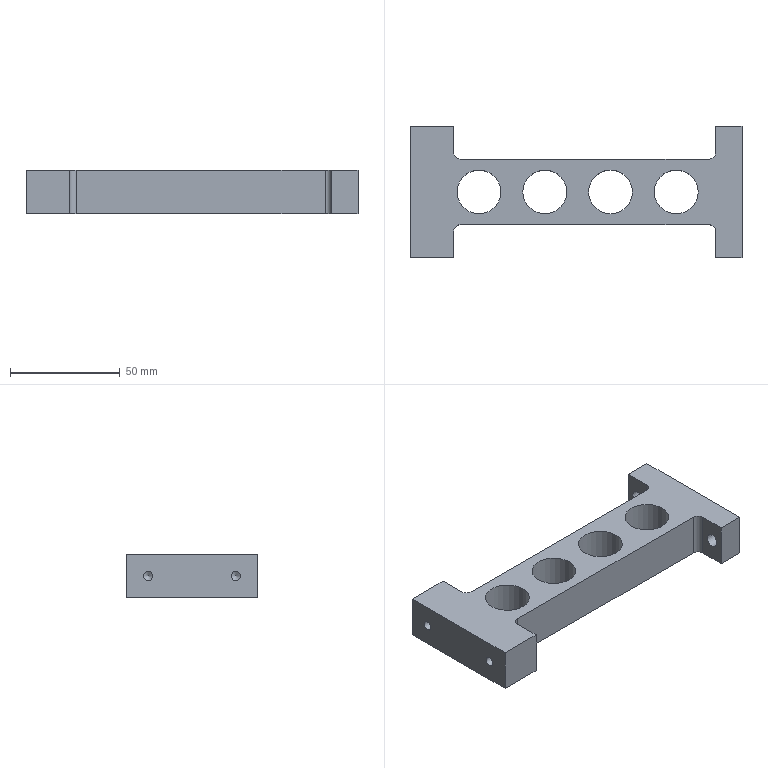Part | NX | 1 solid | 28 faces | box 151.5 x 60 x 20 mm | volume 84044 mm3 | plane 14 | cylinder 12 | cone 2 | commonest cylinder face diameters 6 x6 20 x4 4.2 x2
STEP:
#1=CARTESIAN_POINT('',(-75.75,-30.,-10.));
#2=VERTEX_POINT('',#1);
#3=CARTESIAN_POINT('',(-55.75,-30.,-10.));
#4=VERTEX_POINT('',#3);
#5=CARTESIAN_POINT('',(75.75,-30.,-10.));
#6=DIRECTION('',(1.,0.,0.));
#7=VECTOR('',#6,1000.);
#8=LINE('',#5,#7);
#9=EDGE_CURVE('',#2,#4,#8,.T.);
#10=ORIENTED_EDGE('',*,*,#9,.T.);
#11=CARTESIAN_POINT('',(-55.75,-30.,10.));
#12=VERTEX_POINT('',#11);
#13=CARTESIAN_POINT('',(-55.75,-30.,-10.));
#14=DIRECTION('',(0.,0.,1.));
#15=VECTOR('',#14,1000.);
#16=LINE('',#13,#15);
#17=EDGE_CURVE('',#4,#12,#16,.T.);
#18=ORIENTED_EDGE('',*,*,#17,.T.);
#19=CARTESIAN_POINT('',(-75.75,-30.,10.));
#20=VERTEX_POINT('',#19);
#21=CARTESIAN_POINT('',(75.75,-30.,10.));
#22=DIRECTION('',(1.,0.,0.));
#23=VECTOR('',#22,1000.);
#24=LINE('',#21,#23);
#25=EDGE_CURVE('',#20,#12,#24,.T.);
#26=ORIENTED_EDGE('',*,*,#25,.F.);
#27=CARTESIAN_POINT('',(-75.75,-30.,10.));
#28=DIRECTION('',(0.,0.,-1.));
#29=VECTOR('',#28,1000.);
#30=LINE('',#27,#29);
#31=EDGE_CURVE('',#20,#2,#30,.T.);
#32=ORIENTED_EDGE('',*,*,#31,.T.);
#33=EDGE_LOOP('',(#10,#18,#26,#32));
#34=FACE_BOUND('',#33,.T.);
#35=CARTESIAN_POINT('',(75.75,-30.,10.));
#36=DIRECTION('',(0.,1.,0.));
#37=DIRECTION('',(-1.,0.,0.));
#38=AXIS2_PLACEMENT_3D('',#35,#36,#37);
#39=PLANE('',#38);
#40=ADVANCED_FACE('',(#34),#39,.F.);
#41=CARTESIAN_POINT('',(75.75,30.,-10.));
#42=VERTEX_POINT('',#41);
#43=CARTESIAN_POINT('',(63.75,30.,-10.));
#44=VERTEX_POINT('',#43);
#45=CARTESIAN_POINT('',(75.75,30.,-10.));
#46=DIRECTION('',(-1.,0.,0.));
#47=VECTOR('',#46,1000.);
#48=LINE('',#45,#47);
#49=EDGE_CURVE('',#42,#44,#48,.T.);
#50=ORIENTED_EDGE('',*,*,#49,.T.);
#51=CARTESIAN_POINT('',(63.75,30.,10.));
#52=VERTEX_POINT('',#51);
#53=CARTESIAN_POINT('',(63.75,30.,-10.));
#54=DIRECTION('',(0.,0.,1.));
#55=VECTOR('',#54,1000.);
#56=LINE('',#53,#55);
#57=EDGE_CURVE('',#44,#52,#56,.T.);
#58=ORIENTED_EDGE('',*,*,#57,.T.);
#59=CARTESIAN_POINT('',(75.75,30.,10.));
#60=VERTEX_POINT('',#59);
#61=CARTESIAN_POINT('',(75.75,30.,10.));
#62=DIRECTION('',(-1.,0.,0.));
#63=VECTOR('',#62,1000.);
#64=LINE('',#61,#63);
#65=EDGE_CURVE('',#60,#52,#64,.T.);
#66=ORIENTED_EDGE('',*,*,#65,.F.);
#67=CARTESIAN_POINT('',(75.75,30.,10.));
#68=DIRECTION('',(0.,0.,-1.));
#69=VECTOR('',#68,1000.);
#70=LINE('',#67,#69);
#71=EDGE_CURVE('',#60,#42,#70,.T.);
#72=ORIENTED_EDGE('',*,*,#71,.T.);
#73=EDGE_LOOP('',(#50,#58,#66,#72));
#74=FACE_BOUND('',#73,.T.);
#75=CARTESIAN_POINT('',(75.75,30.,10.));
#76=DIRECTION('',(0.,-1.,0.));
#77=DIRECTION('',(1.,0.,0.));
#78=AXIS2_PLACEMENT_3D('',#75,#76,#77);
#79=PLANE('',#78);
#80=ADVANCED_FACE('',(#74),#79,.F.);
#81=CARTESIAN_POINT('',(-75.75,-20.,2.1));
#82=VERTEX_POINT('',#81);
#83=CARTESIAN_POINT('',(-75.75,-20.,0.));
#84=DIRECTION('',(-1.,0.,0.));
#85=DIRECTION('',(0.,0.,1.));
#86=AXIS2_PLACEMENT_3D('',#83,#84,#85);
#87=CIRCLE('',#86,2.1);
#88=EDGE_CURVE('',#82,#82,#87,.T.);
#89=ORIENTED_EDGE('',*,*,#88,.F.);
#90=EDGE_LOOP('',(#89));
#91=FACE_BOUND('',#90,.T.);
#92=CARTESIAN_POINT('',(-75.75,20.,2.1));
#93=VERTEX_POINT('',#92);
#94=CARTESIAN_POINT('',(-75.75,20.,0.));
#95=DIRECTION('',(-1.,0.,0.));
#96=DIRECTION('',(0.,0.,1.));
#97=AXIS2_PLACEMENT_3D('',#94,#95,#96);
#98=CIRCLE('',#97,2.1);
#99=EDGE_CURVE('',#93,#93,#98,.T.);
#100=ORIENTED_EDGE('',*,*,#99,.F.);
#101=EDGE_LOOP('',(#100));
#102=FACE_BOUND('',#101,.T.);
#103=CARTESIAN_POINT('',(-75.75,30.,-10.));
#104=VERTEX_POINT('',#103);
#105=CARTESIAN_POINT('',(-75.75,30.,-10.));
#106=DIRECTION('',(0.,-1.,0.));
#107=VECTOR('',#106,1000.);
#108=LINE('',#105,#107);
#109=EDGE_CURVE('',#104,#2,#108,.T.);
#110=ORIENTED_EDGE('',*,*,#109,.T.);
#111=ORIENTED_EDGE('',*,*,#31,.F.);
#112=CARTESIAN_POINT('',(-75.75,30.,10.));
#113=VERTEX_POINT('',#112);
#114=CARTESIAN_POINT('',(-75.75,30.,10.));
#115=DIRECTION('',(0.,-1.,0.));
#116=VECTOR('',#115,1000.);
#117=LINE('',#114,#116);
#118=EDGE_CURVE('',#113,#20,#117,.T.);
#119=ORIENTED_EDGE('',*,*,#118,.F.);
#120=CARTESIAN_POINT('',(-75.75,30.,10.));
#121=DIRECTION('',(0.,0.,-1.));
#122=VECTOR('',#121,1000.);
#123=LINE('',#120,#122);
#124=EDGE_CURVE('',#113,#104,#123,.T.);
#125=ORIENTED_EDGE('',*,*,#124,.T.);
#126=EDGE_LOOP('',(#110,#111,#119,#125));
#127=FACE_BOUND('',#126,.T.);
#128=CARTESIAN_POINT('',(-75.75,30.,10.));
#129=DIRECTION('',(1.,0.,0.));
#130=DIRECTION('',(0.,1.,0.));
#131=AXIS2_PLACEMENT_3D('',#128,#129,#130);
#132=PLANE('',#131);
#133=ADVANCED_FACE('',(#91,#102,#127),#132,.F.);
#134=CARTESIAN_POINT('',(63.75,-30.,10.));
#135=VERTEX_POINT('',#134);
#136=CARTESIAN_POINT('',(75.75,-30.,10.));
#137=VERTEX_POINT('',#136);
#138=CARTESIAN_POINT('',(75.75,-30.,10.));
#139=DIRECTION('',(1.,0.,0.));
#140=VECTOR('',#139,1000.);
#141=LINE('',#138,#140);
#142=EDGE_CURVE('',#135,#137,#141,.T.);
#143=ORIENTED_EDGE('',*,*,#142,.F.);
#144=CARTESIAN_POINT('',(63.75,-30.,-10.));
#145=VERTEX_POINT('',#144);
#146=CARTESIAN_POINT('',(63.75,-30.,-10.));
#147=DIRECTION('',(0.,0.,1.));
#148=VECTOR('',#147,1000.);
#149=LINE('',#146,#148);
#150=EDGE_CURVE('',#145,#135,#149,.T.);
#151=ORIENTED_EDGE('',*,*,#150,.F.);
#152=CARTESIAN_POINT('',(75.75,-30.,-10.));
#153=VERTEX_POINT('',#152);
#154=CARTESIAN_POINT('',(75.75,-30.,-10.));
#155=DIRECTION('',(1.,0.,0.));
#156=VECTOR('',#155,1000.);
#157=LINE('',#154,#156);
#158=EDGE_CURVE('',#145,#153,#157,.T.);
#159=ORIENTED_EDGE('',*,*,#158,.T.);
#160=CARTESIAN_POINT('',(75.75,-30.,10.));
#161=DIRECTION('',(0.,0.,-1.));
#162=VECTOR('',#161,1000.);
#163=LINE('',#160,#162);
#164=EDGE_CURVE('',#137,#153,#163,.T.);
#165=ORIENTED_EDGE('',*,*,#164,.F.);
#166=EDGE_LOOP('',(#143,#151,#159,#165));
#167=FACE_BOUND('',#166,.T.);
#168=CARTESIAN_POINT('',(75.75,-30.,10.));
#169=DIRECTION('',(0.,1.,0.));
#170=DIRECTION('',(-1.,0.,0.));
#171=AXIS2_PLACEMENT_3D('',#168,#169,#170);
#172=PLANE('',#171);
#173=ADVANCED_FACE('',(#167),#172,.F.);
#174=CARTESIAN_POINT('',(75.75,-24.,3.));
#175=VERTEX_POINT('',#174);
#176=CARTESIAN_POINT('',(75.75,-24.,0.));
#177=DIRECTION('',(1.,0.,0.));
#178=DIRECTION('',(0.,0.,1.));
#179=AXIS2_PLACEMENT_3D('',#176,#177,#178);
#180=CIRCLE('',#179,3.);
#181=EDGE_CURVE('',#175,#175,#180,.T.);
#182=ORIENTED_EDGE('',*,*,#181,.F.);
#183=EDGE_LOOP('',(#182));
#184=FACE_BOUND('',#183,.T.);
#185=CARTESIAN_POINT('',(75.75,24.,-3.));
#186=VERTEX_POINT('',#185);
#187=CARTESIAN_POINT('',(75.75,24.,0.));
#188=DIRECTION('',(1.,0.,0.));
#189=DIRECTION('',(0.,0.,-1.));
#190=AXIS2_PLACEMENT_3D('',#187,#188,#189);
#191=CIRCLE('',#190,3.);
#192=EDGE_CURVE('',#186,#186,#191,.T.);
#193=ORIENTED_EDGE('',*,*,#192,.F.);
#194=EDGE_LOOP('',(#193));
#195=FACE_BOUND('',#194,.T.);
#196=CARTESIAN_POINT('',(75.75,30.,-10.));
#197=DIRECTION('',(0.,1.,0.));
#198=VECTOR('',#197,1000.);
#199=LINE('',#196,#198);
#200=EDGE_CURVE('',#153,#42,#199,.T.);
#201=ORIENTED_EDGE('',*,*,#200,.T.);
#202=ORIENTED_EDGE('',*,*,#71,.F.);
#203=CARTESIAN_POINT('',(75.75,30.,10.));
#204=DIRECTION('',(0.,1.,0.));
#205=VECTOR('',#204,1000.);
#206=LINE('',#203,#205);
#207=EDGE_CURVE('',#137,#60,#206,.T.);
#208=ORIENTED_EDGE('',*,*,#207,.F.);
#209=ORIENTED_EDGE('',*,*,#164,.T.);
#210=EDGE_LOOP('',(#201,#202,#208,#209));
#211=FACE_BOUND('',#210,.T.);
#212=CARTESIAN_POINT('',(75.75,30.,10.));
#213=DIRECTION('',(-1.,0.,0.));
#214=DIRECTION('',(0.,-1.,0.));
#215=AXIS2_PLACEMENT_3D('',#212,#213,#214);
#216=PLANE('',#215);
#217=ADVANCED_FACE('',(#184,#195,#211),#216,.F.);
#218=CARTESIAN_POINT('',(-55.75,30.,10.));
#219=VERTEX_POINT('',#218);
#220=CARTESIAN_POINT('',(75.75,30.,10.));
#221=DIRECTION('',(-1.,0.,0.));
#222=VECTOR('',#221,1000.);
#223=LINE('',#220,#222);
#224=EDGE_CURVE('',#219,#113,#223,.T.);
#225=ORIENTED_EDGE('',*,*,#224,.F.);
#226=CARTESIAN_POINT('',(-55.75,30.,-10.));
#227=VERTEX_POINT('',#226);
#228=CARTESIAN_POINT('',(-55.75,30.,-10.));
#229=DIRECTION('',(0.,0.,1.));
#230=VECTOR('',#229,1000.);
#231=LINE('',#228,#230);
#232=EDGE_CURVE('',#227,#219,#231,.T.);
#233=ORIENTED_EDGE('',*,*,#232,.F.);
#234=CARTESIAN_POINT('',(75.75,30.,-10.));
#235=DIRECTION('',(-1.,0.,0.));
#236=VECTOR('',#235,1000.);
#237=LINE('',#234,#236);
#238=EDGE_CURVE('',#227,#104,#237,.T.);
#239=ORIENTED_EDGE('',*,*,#238,.T.);
#240=ORIENTED_EDGE('',*,*,#124,.F.);
#241=EDGE_LOOP('',(#225,#233,#239,#240));
#242=FACE_BOUND('',#241,.T.);
#243=CARTESIAN_POINT('',(75.75,30.,10.));
#244=DIRECTION('',(0.,-1.,0.));
#245=DIRECTION('',(1.,0.,0.));
#246=AXIS2_PLACEMENT_3D('',#243,#244,#245);
#247=PLANE('',#246);
#248=ADVANCED_FACE('',(#242),#247,.F.);
#249=CARTESIAN_POINT('',(25.75,0.,10.));
#250=VERTEX_POINT('',#249);
#251=CARTESIAN_POINT('',(15.75,0.,10.));
#252=DIRECTION('',(0.,0.,1.));
#253=DIRECTION('',(1.,0.,0.));
#254=AXIS2_PLACEMENT_3D('',#251,#252,#253);
#255=CIRCLE('',#254,10.);
#256=EDGE_CURVE('',#250,#250,#255,.T.);
#257=ORIENTED_EDGE('',*,*,#256,.F.);
#258=EDGE_LOOP('',(#257));
#259=FACE_BOUND('',#258,.T.);
#260=CARTESIAN_POINT('',(55.75,0.,10.));
#261=VERTEX_POINT('',#260);
#262=CARTESIAN_POINT('',(45.75,0.,10.));
#263=DIRECTION('',(0.,0.,1.));
#264=DIRECTION('',(1.,0.,0.));
#265=AXIS2_PLACEMENT_3D('',#262,#263,#264);
#266=CIRCLE('',#265,10.);
#267=EDGE_CURVE('',#261,#261,#266,.T.);
#268=ORIENTED_EDGE('',*,*,#267,.F.);
#269=EDGE_LOOP('',(#268));
#270=FACE_BOUND('',#269,.T.);
#271=ORIENTED_EDGE('',*,*,#25,.T.);
#272=CARTESIAN_POINT('',(-55.75,-18.,10.));
#273=VERTEX_POINT('',#272);
#274=CARTESIAN_POINT('',(-55.75,-30.,10.));
#275=DIRECTION('',(0.,-1.,0.));
#276=VECTOR('',#275,1000.);
#277=LINE('',#274,#276);
#278=EDGE_CURVE('',#273,#12,#277,.T.);
#279=ORIENTED_EDGE('',*,*,#278,.F.);
#280=CARTESIAN_POINT('',(-52.75,-15.,10.));
#281=VERTEX_POINT('',#280);
#282=CARTESIAN_POINT('',(-52.75,-18.,10.));
#283=DIRECTION('',(0.,0.,-1.));
#284=DIRECTION('',(-1.,0.,0.));
#285=AXIS2_PLACEMENT_3D('',#282,#283,#284);
#286=CIRCLE('',#285,3.);
#287=EDGE_CURVE('',#273,#281,#286,.T.);
#288=ORIENTED_EDGE('',*,*,#287,.T.);
#289=CARTESIAN_POINT('',(60.75,-15.,10.));
#290=VERTEX_POINT('',#289);
#291=CARTESIAN_POINT('',(63.75,-15.,10.));
#292=DIRECTION('',(-1.,0.,0.));
#293=VECTOR('',#292,1000.);
#294=LINE('',#291,#293);
#295=EDGE_CURVE('',#290,#281,#294,.T.);
#296=ORIENTED_EDGE('',*,*,#295,.F.);
#297=CARTESIAN_POINT('',(63.75,-18.,10.));
#298=VERTEX_POINT('',#297);
#299=CARTESIAN_POINT('',(60.75,-18.,10.));
#300=DIRECTION('',(0.,0.,-1.));
#301=DIRECTION('',(-1.,0.,0.));
#302=AXIS2_PLACEMENT_3D('',#299,#300,#301);
#303=CIRCLE('',#302,3.);
#304=EDGE_CURVE('',#290,#298,#303,.T.);
#305=ORIENTED_EDGE('',*,*,#304,.T.);
#306=CARTESIAN_POINT('',(63.75,-30.,10.));
#307=DIRECTION('',(0.,1.,0.));
#308=VECTOR('',#307,1000.);
#309=LINE('',#306,#308);
#310=EDGE_CURVE('',#135,#298,#309,.T.);
#311=ORIENTED_EDGE('',*,*,#310,.F.);
#312=ORIENTED_EDGE('',*,*,#142,.T.);
#313=ORIENTED_EDGE('',*,*,#207,.T.);
#314=ORIENTED_EDGE('',*,*,#65,.T.);
#315=CARTESIAN_POINT('',(63.75,18.,10.));
#316=VERTEX_POINT('',#315);
#317=CARTESIAN_POINT('',(63.75,30.,10.));
#318=DIRECTION('',(0.,1.,0.));
#319=VECTOR('',#318,1000.);
#320=LINE('',#317,#319);
#321=EDGE_CURVE('',#316,#52,#320,.T.);
#322=ORIENTED_EDGE('',*,*,#321,.F.);
#323=CARTESIAN_POINT('',(60.75,15.,10.));
#324=VERTEX_POINT('',#323);
#325=CARTESIAN_POINT('',(60.75,18.,10.));
#326=DIRECTION('',(0.,0.,-1.));
#327=DIRECTION('',(-1.,0.,0.));
#328=AXIS2_PLACEMENT_3D('',#325,#326,#327);
#329=CIRCLE('',#328,3.);
#330=EDGE_CURVE('',#316,#324,#329,.T.);
#331=ORIENTED_EDGE('',*,*,#330,.T.);
#332=CARTESIAN_POINT('',(-52.75,15.,10.));
#333=VERTEX_POINT('',#332);
#334=CARTESIAN_POINT('',(63.75,15.,10.));
#335=DIRECTION('',(1.,0.,0.));
#336=VECTOR('',#335,1000.);
#337=LINE('',#334,#336);
#338=EDGE_CURVE('',#333,#324,#337,.T.);
#339=ORIENTED_EDGE('',*,*,#338,.F.);
#340=CARTESIAN_POINT('',(-55.75,18.,10.));
#341=VERTEX_POINT('',#340);
#342=CARTESIAN_POINT('',(-52.75,18.,10.));
#343=DIRECTION('',(0.,0.,-1.));
#344=DIRECTION('',(-1.,0.,0.));
#345=AXIS2_PLACEMENT_3D('',#342,#343,#344);
#346=CIRCLE('',#345,3.);
#347=EDGE_CURVE('',#333,#341,#346,.T.);
#348=ORIENTED_EDGE('',*,*,#347,.T.);
#349=CARTESIAN_POINT('',(-55.75,30.,10.));
#350=DIRECTION('',(0.,-1.,0.));
#351=VECTOR('',#350,1000.);
#352=LINE('',#349,#351);
#353=EDGE_CURVE('',#219,#341,#352,.T.);
#354=ORIENTED_EDGE('',*,*,#353,.F.);
#355=ORIENTED_EDGE('',*,*,#224,.T.);
#356=ORIENTED_EDGE('',*,*,#118,.T.);
#357=EDGE_LOOP('',(#271,#279,#288,#296,#305,#311,#312,#313,#314,#322,#331,#339,#348,#354,#355,#356));
#358=FACE_BOUND('',#357,.T.);
#359=CARTESIAN_POINT('',(-4.25,0.,10.));
#360=VERTEX_POINT('',#359);
#361=CARTESIAN_POINT('',(-14.25,0.,10.));
#362=DIRECTION('',(0.,0.,1.));
#363=DIRECTION('',(1.,0.,0.));
#364=AXIS2_PLACEMENT_3D('',#361,#362,#363);
#365=CIRCLE('',#364,10.);
#366=EDGE_CURVE('',#360,#360,#365,.T.);
#367=ORIENTED_EDGE('',*,*,#366,.F.);
#368=EDGE_LOOP('',(#367));
#369=FACE_BOUND('',#368,.T.);
#370=CARTESIAN_POINT('',(-34.25,0.,10.));
#371=VERTEX_POINT('',#370);
#372=CARTESIAN_POINT('',(-44.25,0.,10.));
#373=DIRECTION('',(0.,0.,1.));
#374=DIRECTION('',(1.,0.,0.));
#375=AXIS2_PLACEMENT_3D('',#372,#373,#374);
#376=CIRCLE('',#375,10.);
#377=EDGE_CURVE('',#371,#371,#376,.T.);
#378=ORIENTED_EDGE('',*,*,#377,.F.);
#379=EDGE_LOOP('',(#378));
#380=FACE_BOUND('',#379,.T.);
#381=CARTESIAN_POINT('',(0.,0.,10.));
#382=DIRECTION('',(0.,0.,-1.));
#383=DIRECTION('',(-1.,0.,0.));
#384=AXIS2_PLACEMENT_3D('',#381,#382,#383);
#385=PLANE('',#384);
#386=ADVANCED_FACE('',(#259,#270,#358,#369,#380),#385,.F.);
#387=CARTESIAN_POINT('',(60.75,-15.,-10.));
#388=VERTEX_POINT('',#387);
#389=CARTESIAN_POINT('',(-52.75,-15.,-10.));
#390=VERTEX_POINT('',#389);
#391=CARTESIAN_POINT('',(63.75,-15.,-10.));
#392=DIRECTION('',(-1.,0.,0.));
#393=VECTOR('',#392,1000.);
#394=LINE('',#391,#393);
#395=EDGE_CURVE('',#388,#390,#394,.T.);
#396=ORIENTED_EDGE('',*,*,#395,.T.);
#397=CARTESIAN_POINT('',(-55.75,-18.,-10.));
#398=VERTEX_POINT('',#397);
#399=CARTESIAN_POINT('',(-52.75,-18.,-10.));
#400=DIRECTION('',(0.,0.,-1.));
#401=DIRECTION('',(-1.,0.,0.));
#402=AXIS2_PLACEMENT_3D('',#399,#400,#401);
#403=CIRCLE('',#402,3.);
#404=EDGE_CURVE('',#390,#398,#403,.F.);
#405=ORIENTED_EDGE('',*,*,#404,.T.);
#406=CARTESIAN_POINT('',(-55.75,-30.,-10.));
#407=DIRECTION('',(0.,-1.,0.));
#408=VECTOR('',#407,1000.);
#409=LINE('',#406,#408);
#410=EDGE_CURVE('',#398,#4,#409,.T.);
#411=ORIENTED_EDGE('',*,*,#410,.T.);
#412=ORIENTED_EDGE('',*,*,#9,.F.);
#413=ORIENTED_EDGE('',*,*,#109,.F.);
#414=ORIENTED_EDGE('',*,*,#238,.F.);
#415=CARTESIAN_POINT('',(-55.75,18.,-10.));
#416=VERTEX_POINT('',#415);
#417=CARTESIAN_POINT('',(-55.75,30.,-10.));
#418=DIRECTION('',(0.,-1.,0.));
#419=VECTOR('',#418,1000.);
#420=LINE('',#417,#419);
#421=EDGE_CURVE('',#227,#416,#420,.T.);
#422=ORIENTED_EDGE('',*,*,#421,.T.);
#423=CARTESIAN_POINT('',(-52.75,15.,-10.));
#424=VERTEX_POINT('',#423);
#425=CARTESIAN_POINT('',(-52.75,18.,-10.));
#426=DIRECTION('',(0.,0.,-1.));
#427=DIRECTION('',(-1.,0.,0.));
#428=AXIS2_PLACEMENT_3D('',#425,#426,#427);
#429=CIRCLE('',#428,3.);
#430=EDGE_CURVE('',#416,#424,#429,.F.);
#431=ORIENTED_EDGE('',*,*,#430,.T.);
#432=CARTESIAN_POINT('',(60.75,15.,-10.));
#433=VERTEX_POINT('',#432);
#434=CARTESIAN_POINT('',(63.75,15.,-10.));
#435=DIRECTION('',(1.,0.,0.));
#436=VECTOR('',#435,1000.);
#437=LINE('',#434,#436);
#438=EDGE_CURVE('',#424,#433,#437,.T.);
#439=ORIENTED_EDGE('',*,*,#438,.T.);
#440=CARTESIAN_POINT('',(63.75,18.,-10.));
#441=VERTEX_POINT('',#440);
#442=CARTESIAN_POINT('',(60.75,18.,-10.));
#443=DIRECTION('',(0.,0.,-1.));
#444=DIRECTION('',(-1.,0.,0.));
#445=AXIS2_PLACEMENT_3D('',#442,#443,#444);
#446=CIRCLE('',#445,3.);
#447=EDGE_CURVE('',#433,#441,#446,.F.);
#448=ORIENTED_EDGE('',*,*,#447,.T.);
#449=CARTESIAN_POINT('',(63.75,30.,-10.));
#450=DIRECTION('',(0.,1.,0.));
#451=VECTOR('',#450,1000.);
#452=LINE('',#449,#451);
#453=EDGE_CURVE('',#441,#44,#452,.T.);
#454=ORIENTED_EDGE('',*,*,#453,.T.);
#455=ORIENTED_EDGE('',*,*,#49,.F.);
#456=ORIENTED_EDGE('',*,*,#200,.F.);
#457=ORIENTED_EDGE('',*,*,#158,.F.);
#458=CARTESIAN_POINT('',(63.75,-18.,-10.));
#459=VERTEX_POINT('',#458);
#460=CARTESIAN_POINT('',(63.75,-30.,-10.));
#461=DIRECTION('',(0.,1.,0.));
#462=VECTOR('',#461,1000.);
#463=LINE('',#460,#462);
#464=EDGE_CURVE('',#145,#459,#463,.T.);
#465=ORIENTED_EDGE('',*,*,#464,.T.);
#466=CARTESIAN_POINT('',(60.75,-18.,-10.));
#467=DIRECTION('',(0.,0.,-1.));
#468=DIRECTION('',(-1.,0.,0.));
#469=AXIS2_PLACEMENT_3D('',#466,#467,#468);
#470=CIRCLE('',#469,3.);
#471=EDGE_CURVE('',#459,#388,#470,.F.);
#472=ORIENTED_EDGE('',*,*,#471,.T.);
#473=EDGE_LOOP('',(#396,#405,#411,#412,#413,#414,#422,#431,#439,#448,#454,#455,#456,#457,#465,#472));
#474=FACE_BOUND('',#473,.T.);
#475=CARTESIAN_POINT('',(5.75,0.,-10.));
#476=VERTEX_POINT('',#475);
#477=CARTESIAN_POINT('',(15.75,0.,-10.));
#478=DIRECTION('',(0.,0.,-1.));
#479=DIRECTION('',(-1.,0.,0.));
#480=AXIS2_PLACEMENT_3D('',#477,#478,#479);
#481=CIRCLE('',#480,10.);
#482=EDGE_CURVE('',#476,#476,#481,.T.);
#483=ORIENTED_EDGE('',*,*,#482,.F.);
#484=EDGE_LOOP('',(#483));
#485=FACE_BOUND('',#484,.T.);
#486=CARTESIAN_POINT('',(35.75,0.,-10.));
#487=VERTEX_POINT('',#486);
#488=CARTESIAN_POINT('',(45.75,0.,-10.));
#489=DIRECTION('',(0.,0.,-1.));
#490=DIRECTION('',(-1.,0.,0.));
#491=AXIS2_PLACEMENT_3D('',#488,#489,#490);
#492=CIRCLE('',#491,10.);
#493=EDGE_CURVE('',#487,#487,#492,.T.);
#494=ORIENTED_EDGE('',*,*,#493,.F.);
#495=EDGE_LOOP('',(#494));
#496=FACE_BOUND('',#495,.T.);
#497=CARTESIAN_POINT('',(-24.25,0.,-10.));
#498=VERTEX_POINT('',#497);
#499=CARTESIAN_POINT('',(-14.25,0.,-10.));
#500=DIRECTION('',(0.,0.,-1.));
#501=DIRECTION('',(-1.,0.,0.));
#502=AXIS2_PLACEMENT_3D('',#499,#500,#501);
#503=CIRCLE('',#502,10.);
#504=EDGE_CURVE('',#498,#498,#503,.T.);
#505=ORIENTED_EDGE('',*,*,#504,.F.);
#506=EDGE_LOOP('',(#505));
#507=FACE_BOUND('',#506,.T.);
#508=CARTESIAN_POINT('',(-54.25,0.,-10.));
#509=VERTEX_POINT('',#508);
#510=CARTESIAN_POINT('',(-44.25,0.,-10.));
#511=DIRECTION('',(0.,0.,-1.));
#512=DIRECTION('',(-1.,0.,0.));
#513=AXIS2_PLACEMENT_3D('',#510,#511,#512);
#514=CIRCLE('',#513,10.);
#515=EDGE_CURVE('',#509,#509,#514,.T.);
#516=ORIENTED_EDGE('',*,*,#515,.F.);
#517=EDGE_LOOP('',(#516));
#518=FACE_BOUND('',#517,.T.);
#519=CARTESIAN_POINT('',(0.,0.,-10.));
#520=DIRECTION('',(0.,0.,-1.));
#521=DIRECTION('',(-1.,0.,0.));
#522=AXIS2_PLACEMENT_3D('',#519,#520,#521);
#523=PLANE('',#522);
#524=ADVANCED_FACE('',(#474,#485,#496,#507,#518),#523,.T.);
#525=ORIENTED_EDGE('',*,*,#493,.T.);
#526=EDGE_LOOP('',(#525));
#527=FACE_BOUND('',#526,.T.);
#528=ORIENTED_EDGE('',*,*,#267,.T.);
#529=EDGE_LOOP('',(#528));
#530=FACE_BOUND('',#529,.T.);
#531=CARTESIAN_POINT('',(45.75,0.,-15.));
#532=DIRECTION('',(0.,0.,1.));
#533=DIRECTION('',(1.,0.,0.));
#534=AXIS2_PLACEMENT_3D('',#531,#532,#533);
#535=CYLINDRICAL_SURFACE('',#534,10.);
#536=ADVANCED_FACE('',(#527,#530),#535,.F.);
#537=ORIENTED_EDGE('',*,*,#482,.T.);
#538=EDGE_LOOP('',(#537));
#539=FACE_BOUND('',#538,.T.);
#540=ORIENTED_EDGE('',*,*,#256,.T.);
#541=EDGE_LOOP('',(#540));
#542=FACE_BOUND('',#541,.T.);
#543=CARTESIAN_POINT('',(15.75,0.,-15.));
#544=DIRECTION('',(0.,0.,1.));
#545=DIRECTION('',(1.,0.,0.));
#546=AXIS2_PLACEMENT_3D('',#543,#544,#545);
#547=CYLINDRICAL_SURFACE('',#546,10.);
#548=ADVANCED_FACE('',(#539,#542),#547,.F.);
#549=ORIENTED_EDGE('',*,*,#504,.T.);
#550=EDGE_LOOP('',(#549));
#551=FACE_BOUND('',#550,.T.);
#552=ORIENTED_EDGE('',*,*,#366,.T.);
#553=EDGE_LOOP('',(#552));
#554=FACE_BOUND('',#553,.T.);
#555=CARTESIAN_POINT('',(-14.25,0.,-15.));
#556=DIRECTION('',(0.,0.,1.));
#557=DIRECTION('',(1.,0.,0.));
#558=AXIS2_PLACEMENT_3D('',#555,#556,#557);
#559=CYLINDRICAL_SURFACE('',#558,10.);
#560=ADVANCED_FACE('',(#551,#554),#559,.F.);
#561=ORIENTED_EDGE('',*,*,#515,.T.);
#562=EDGE_LOOP('',(#561));
#563=FACE_BOUND('',#562,.T.);
#564=ORIENTED_EDGE('',*,*,#377,.T.);
#565=EDGE_LOOP('',(#564));
#566=FACE_BOUND('',#565,.T.);
#567=CARTESIAN_POINT('',(-44.25,0.,-15.));
#568=DIRECTION('',(0.,0.,1.));
#569=DIRECTION('',(1.,0.,0.));
#570=AXIS2_PLACEMENT_3D('',#567,#568,#569);
#571=CYLINDRICAL_SURFACE('',#570,10.);
#572=ADVANCED_FACE('',(#563,#566),#571,.F.);
#573=CARTESIAN_POINT('',(63.75,24.,-3.));
#574=VERTEX_POINT('',#573);
#575=CARTESIAN_POINT('',(63.75,24.,0.));
#576=DIRECTION('',(1.,0.,0.));
#577=DIRECTION('',(0.,0.,-1.));
#578=AXIS2_PLACEMENT_3D('',#575,#576,#577);
#579=CIRCLE('',#578,3.);
#580=EDGE_CURVE('',#574,#574,#579,.T.);
#581=ORIENTED_EDGE('',*,*,#580,.T.);
#582=EDGE_LOOP('',(#581));
#583=FACE_BOUND('',#582,.T.);
#584=ORIENTED_EDGE('',*,*,#453,.F.);
#585=CARTESIAN_POINT('',(63.75,18.,10.));
#586=DIRECTION('',(0.,0.,1.));
#587=VECTOR('',#586,1000.);
#588=LINE('',#585,#587);
#589=EDGE_CURVE('',#441,#316,#588,.T.);
#590=ORIENTED_EDGE('',*,*,#589,.T.);
#591=ORIENTED_EDGE('',*,*,#321,.T.);
#592=ORIENTED_EDGE('',*,*,#57,.F.);
#593=EDGE_LOOP('',(#584,#590,#591,#592));
#594=FACE_BOUND('',#593,.T.);
#595=CARTESIAN_POINT('',(63.75,30.,-10.));
#596=DIRECTION('',(1.,0.,0.));
#597=DIRECTION('',(0.,0.,-1.));
#598=AXIS2_PLACEMENT_3D('',#595,#596,#597);
#599=PLANE('',#598);
#600=ADVANCED_FACE('',(#583,#594),#599,.F.);
#601=ORIENTED_EDGE('',*,*,#438,.F.);
#602=CARTESIAN_POINT('',(-52.75,15.,10.));
#603=DIRECTION('',(0.,0.,1.));
#604=VECTOR('',#603,1000.);
#605=LINE('',#602,#604);
#606=EDGE_CURVE('',#424,#333,#605,.T.);
#607=ORIENTED_EDGE('',*,*,#606,.T.);
#608=ORIENTED_EDGE('',*,*,#338,.T.);
#609=CARTESIAN_POINT('',(60.75,15.,-10.));
#610=DIRECTION('',(0.,0.,1.));
#611=VECTOR('',#610,1000.);
#612=LINE('',#609,#611);
#613=EDGE_CURVE('',#324,#433,#612,.F.);
#614=ORIENTED_EDGE('',*,*,#613,.T.);
#615=EDGE_LOOP('',(#601,#607,#608,#614));
#616=FACE_BOUND('',#615,.T.);
#617=CARTESIAN_POINT('',(63.75,15.,-10.));
#618=DIRECTION('',(0.,-1.,0.));
#619=DIRECTION('',(1.,0.,0.));
#620=AXIS2_PLACEMENT_3D('',#617,#618,#619);
#621=PLANE('',#620);
#622=ADVANCED_FACE('',(#616),#621,.F.);
#623=ORIENTED_EDGE('',*,*,#353,.T.);
#624=CARTESIAN_POINT('',(-55.75,18.,-10.));
#625=DIRECTION('',(0.,0.,1.));
#626=VECTOR('',#625,1000.);
#627=LINE('',#624,#626);
#628=EDGE_CURVE('',#341,#416,#627,.F.);
#629=ORIENTED_EDGE('',*,*,#628,.T.);
#630=ORIENTED_EDGE('',*,*,#421,.F.);
#631=ORIENTED_EDGE('',*,*,#232,.T.);
#632=EDGE_LOOP('',(#623,#629,#630,#631));
#633=FACE_BOUND('',#632,.T.);
#634=CARTESIAN_POINT('',(-55.75,30.,-10.));
#635=DIRECTION('',(-1.,0.,0.));
#636=DIRECTION('',(0.,0.,1.));
#637=AXIS2_PLACEMENT_3D('',#634,#635,#636);
#638=PLANE('',#637);
#639=ADVANCED_FACE('',(#633),#638,.F.);
#640=ORIENTED_EDGE('',*,*,#410,.F.);
#641=CARTESIAN_POINT('',(-55.75,-18.,10.));
#642=DIRECTION('',(0.,0.,1.));
#643=VECTOR('',#642,1000.);
#644=LINE('',#641,#643);
#645=EDGE_CURVE('',#398,#273,#644,.T.);
#646=ORIENTED_EDGE('',*,*,#645,.T.);
#647=ORIENTED_EDGE('',*,*,#278,.T.);
#648=ORIENTED_EDGE('',*,*,#17,.F.);
#649=EDGE_LOOP('',(#640,#646,#647,#648));
#650=FACE_BOUND('',#649,.T.);
#651=CARTESIAN_POINT('',(-55.75,-30.,-10.));
#652=DIRECTION('',(-1.,0.,0.));
#653=DIRECTION('',(0.,0.,1.));
#654=AXIS2_PLACEMENT_3D('',#651,#652,#653);
#655=PLANE('',#654);
#656=ADVANCED_FACE('',(#650),#655,.F.);
#657=ORIENTED_EDGE('',*,*,#295,.T.);
#658=CARTESIAN_POINT('',(-52.75,-15.,-10.));
#659=DIRECTION('',(0.,0.,1.));
#660=VECTOR('',#659,1000.);
#661=LINE('',#658,#660);
#662=EDGE_CURVE('',#281,#390,#661,.F.);
#663=ORIENTED_EDGE('',*,*,#662,.T.);
#664=ORIENTED_EDGE('',*,*,#395,.F.);
#665=CARTESIAN_POINT('',(60.75,-15.,10.));
#666=DIRECTION('',(0.,0.,1.));
#667=VECTOR('',#666,1000.);
#668=LINE('',#665,#667);
#669=EDGE_CURVE('',#388,#290,#668,.T.);
#670=ORIENTED_EDGE('',*,*,#669,.T.);
#671=EDGE_LOOP('',(#657,#663,#664,#670));
#672=FACE_BOUND('',#671,.T.);
#673=CARTESIAN_POINT('',(63.75,-15.,-10.));
#674=DIRECTION('',(0.,1.,0.));
#675=DIRECTION('',(-1.,0.,0.));
#676=AXIS2_PLACEMENT_3D('',#673,#674,#675);
#677=PLANE('',#676);
#678=ADVANCED_FACE('',(#672),#677,.F.);
#679=CARTESIAN_POINT('',(63.75,-24.,-3.));
#680=VERTEX_POINT('',#679);
#681=CARTESIAN_POINT('',(63.75,-24.,0.));
#682=DIRECTION('',(1.,0.,0.));
#683=DIRECTION('',(0.,0.,-1.));
#684=AXIS2_PLACEMENT_3D('',#681,#682,#683);
#685=CIRCLE('',#684,3.);
#686=EDGE_CURVE('',#680,#680,#685,.T.);
#687=ORIENTED_EDGE('',*,*,#686,.T.);
#688=EDGE_LOOP('',(#687));
#689=FACE_BOUND('',#688,.T.);
#690=ORIENTED_EDGE('',*,*,#310,.T.);
#691=CARTESIAN_POINT('',(63.75,-18.,-10.));
#692=DIRECTION('',(0.,0.,1.));
#693=VECTOR('',#692,1000.);
#694=LINE('',#691,#693);
#695=EDGE_CURVE('',#298,#459,#694,.F.);
#696=ORIENTED_EDGE('',*,*,#695,.T.);
#697=ORIENTED_EDGE('',*,*,#464,.F.);
#698=ORIENTED_EDGE('',*,*,#150,.T.);
#699=EDGE_LOOP('',(#690,#696,#697,#698));
#700=FACE_BOUND('',#699,.T.);
#701=CARTESIAN_POINT('',(63.75,-30.,-10.));
#702=DIRECTION('',(1.,0.,0.));
#703=DIRECTION('',(0.,0.,-1.));
#704=AXIS2_PLACEMENT_3D('',#701,#702,#703);
#705=PLANE('',#704);
#706=ADVANCED_FACE('',(#689,#700),#705,.F.);
#707=ORIENTED_EDGE('',*,*,#192,.T.);
#708=EDGE_LOOP('',(#707));
#709=FACE_BOUND('',#708,.T.);
#710=ORIENTED_EDGE('',*,*,#580,.F.);
#711=EDGE_LOOP('',(#710));
#712=FACE_BOUND('',#711,.T.);
#713=CARTESIAN_POINT('',(55.75,24.,0.));
#714=DIRECTION('',(1.,0.,0.));
#715=DIRECTION('',(0.,0.,-1.));
#716=AXIS2_PLACEMENT_3D('',#713,#714,#715);
#717=CYLINDRICAL_SURFACE('',#716,3.);
#718=ADVANCED_FACE('',(#709,#712),#717,.F.);
#719=ORIENTED_EDGE('',*,*,#181,.T.);
#720=EDGE_LOOP('',(#719));
#721=FACE_BOUND('',#720,.T.);
#722=ORIENTED_EDGE('',*,*,#686,.F.);
#723=EDGE_LOOP('',(#722));
#724=FACE_BOUND('',#723,.T.);
#725=CARTESIAN_POINT('',(55.75,-24.,0.));
#726=DIRECTION('',(1.,0.,0.));
#727=DIRECTION('',(0.,0.,-1.));
#728=AXIS2_PLACEMENT_3D('',#725,#726,#727);
#729=CYLINDRICAL_SURFACE('',#728,3.);
#730=ADVANCED_FACE('',(#721,#724),#729,.F.);
#731=CARTESIAN_POINT('',(-60.488,20.,0.));
#732=VERTEX_POINT('',#731);
#733=VERTEX_LOOP('',#732);
#734=FACE_BOUND('',#733,.T.);
#735=CARTESIAN_POINT('',(-61.75,20.,2.1));
#736=VERTEX_POINT('',#735);
#737=CARTESIAN_POINT('',(-61.75,20.,0.));
#738=DIRECTION('',(-1.,0.,0.));
#739=DIRECTION('',(0.,0.,1.));
#740=AXIS2_PLACEMENT_3D('',#737,#738,#739);
#741=CIRCLE('',#740,2.1);
#742=EDGE_CURVE('',#736,#736,#741,.T.);
#743=ORIENTED_EDGE('',*,*,#742,.T.);
#744=EDGE_LOOP('',(#743));
#745=FACE_BOUND('',#744,.T.);
#746=CARTESIAN_POINT('',(-61.75,20.,0.));
#747=DIRECTION('',(-1.,0.,0.));
#748=DIRECTION('',(0.,0.,1.));
#749=AXIS2_PLACEMENT_3D('',#746,#747,#748);
#750=CONICAL_SURFACE('',#749,2.1,1.03);
#751=ADVANCED_FACE('',(#734,#745),#750,.F.);
#752=ORIENTED_EDGE('',*,*,#742,.F.);
#753=EDGE_LOOP('',(#752));
#754=FACE_BOUND('',#753,.T.);
#755=ORIENTED_EDGE('',*,*,#99,.T.);
#756=EDGE_LOOP('',(#755));
#757=FACE_BOUND('',#756,.T.);
#758=CARTESIAN_POINT('',(-75.75,20.,0.));
#759=DIRECTION('',(-1.,0.,0.));
#760=DIRECTION('',(0.,0.,1.));
#761=AXIS2_PLACEMENT_3D('',#758,#759,#760);
#762=CYLINDRICAL_SURFACE('',#761,2.1);
#763=ADVANCED_FACE('',(#754,#757),#762,.F.);
#764=CARTESIAN_POINT('',(-60.488,-20.,0.));
#765=VERTEX_POINT('',#764);
#766=VERTEX_LOOP('',#765);
#767=FACE_BOUND('',#766,.T.);
#768=CARTESIAN_POINT('',(-61.75,-20.,2.1));
#769=VERTEX_POINT('',#768);
#770=CARTESIAN_POINT('',(-61.75,-20.,0.));
#771=DIRECTION('',(-1.,0.,0.));
#772=DIRECTION('',(0.,0.,1.));
#773=AXIS2_PLACEMENT_3D('',#770,#771,#772);
#774=CIRCLE('',#773,2.1);
#775=EDGE_CURVE('',#769,#769,#774,.T.);
#776=ORIENTED_EDGE('',*,*,#775,.T.);
#777=EDGE_LOOP('',(#776));
#778=FACE_BOUND('',#777,.T.);
#779=CARTESIAN_POINT('',(-61.75,-20.,0.));
#780=DIRECTION('',(-1.,0.,0.));
#781=DIRECTION('',(0.,0.,1.));
#782=AXIS2_PLACEMENT_3D('',#779,#780,#781);
#783=CONICAL_SURFACE('',#782,2.1,1.03);
#784=ADVANCED_FACE('',(#767,#778),#783,.F.);
#785=ORIENTED_EDGE('',*,*,#775,.F.);
#786=EDGE_LOOP('',(#785));
#787=FACE_BOUND('',#786,.T.);
#788=ORIENTED_EDGE('',*,*,#88,.T.);
#789=EDGE_LOOP('',(#788));
#790=FACE_BOUND('',#789,.T.);
#791=CARTESIAN_POINT('',(-75.75,-20.,0.));
#792=DIRECTION('',(-1.,0.,0.));
#793=DIRECTION('',(0.,0.,1.));
#794=AXIS2_PLACEMENT_3D('',#791,#792,#793);
#795=CYLINDRICAL_SURFACE('',#794,2.1);
#796=ADVANCED_FACE('',(#787,#790),#795,.F.);
#797=ORIENTED_EDGE('',*,*,#404,.F.);
#798=ORIENTED_EDGE('',*,*,#662,.F.);
#799=ORIENTED_EDGE('',*,*,#287,.F.);
#800=ORIENTED_EDGE('',*,*,#645,.F.);
#801=EDGE_LOOP('',(#797,#798,#799,#800));
#802=FACE_BOUND('',#801,.T.);
#803=CARTESIAN_POINT('',(-52.75,-18.,-10.));
#804=DIRECTION('',(0.,0.,-1.));
#805=DIRECTION('',(-1.,0.,0.));
#806=AXIS2_PLACEMENT_3D('',#803,#804,#805);
#807=CYLINDRICAL_SURFACE('',#806,3.);
#808=ADVANCED_FACE('',(#802),#807,.F.);
#809=ORIENTED_EDGE('',*,*,#430,.F.);
#810=ORIENTED_EDGE('',*,*,#628,.F.);
#811=ORIENTED_EDGE('',*,*,#347,.F.);
#812=ORIENTED_EDGE('',*,*,#606,.F.);
#813=EDGE_LOOP('',(#809,#810,#811,#812));
#814=FACE_BOUND('',#813,.T.);
#815=CARTESIAN_POINT('',(-52.75,18.,-10.));
#816=DIRECTION('',(0.,0.,-1.));
#817=DIRECTION('',(-1.,0.,0.));
#818=AXIS2_PLACEMENT_3D('',#815,#816,#817);
#819=CYLINDRICAL_SURFACE('',#818,3.);
#820=ADVANCED_FACE('',(#814),#819,.F.);
#821=ORIENTED_EDGE('',*,*,#471,.F.);
#822=ORIENTED_EDGE('',*,*,#695,.F.);
#823=ORIENTED_EDGE('',*,*,#304,.F.);
#824=ORIENTED_EDGE('',*,*,#669,.F.);
#825=EDGE_LOOP('',(#821,#822,#823,#824));
#826=FACE_BOUND('',#825,.T.);
#827=CARTESIAN_POINT('',(60.75,-18.,-10.));
#828=DIRECTION('',(0.,0.,-1.));
#829=DIRECTION('',(-1.,0.,0.));
#830=AXIS2_PLACEMENT_3D('',#827,#828,#829);
#831=CYLINDRICAL_SURFACE('',#830,3.);
#832=ADVANCED_FACE('',(#826),#831,.F.);
#833=ORIENTED_EDGE('',*,*,#447,.F.);
#834=ORIENTED_EDGE('',*,*,#613,.F.);
#835=ORIENTED_EDGE('',*,*,#330,.F.);
#836=ORIENTED_EDGE('',*,*,#589,.F.);
#837=EDGE_LOOP('',(#833,#834,#835,#836));
#838=FACE_BOUND('',#837,.T.);
#839=CARTESIAN_POINT('',(60.75,18.,-10.));
#840=DIRECTION('',(0.,0.,-1.));
#841=DIRECTION('',(-1.,0.,0.));
#842=AXIS2_PLACEMENT_3D('',#839,#840,#841);
#843=CYLINDRICAL_SURFACE('',#842,3.);
#844=ADVANCED_FACE('',(#838),#843,.F.);
#845=CLOSED_SHELL('',(#40,#80,#133,#173,#217,#248,#386,#524,#536,#548,#560,#572,#600,#622,#639,#656,#678,#706,#718,#730,#751,#763,#784,#796,#808,#820,#832,#844));
#846=MANIFOLD_SOLID_BREP('',#845);
#847=(LENGTH_UNIT()NAMED_UNIT(*)SI_UNIT(.MILLI.,.METRE.));
#848=UNCERTAINTY_MEASURE_WITH_UNIT(LENGTH_MEASURE(0.00001),#847,'','');
#849=(NAMED_UNIT(*)PLANE_ANGLE_UNIT()SI_UNIT($,.RADIAN.));
#850=(NAMED_UNIT(*)SI_UNIT($,.STERADIAN.)SOLID_ANGLE_UNIT());
#851=(GEOMETRIC_REPRESENTATION_CONTEXT(3)GLOBAL_UNCERTAINTY_ASSIGNED_CONTEXT((#848))GLOBAL_UNIT_ASSIGNED_CONTEXT((#847,#849,#850))REPRESENTATION_CONTEXT('',''));
#852=ADVANCED_BREP_SHAPE_REPRESENTATION('',(#846),#851);